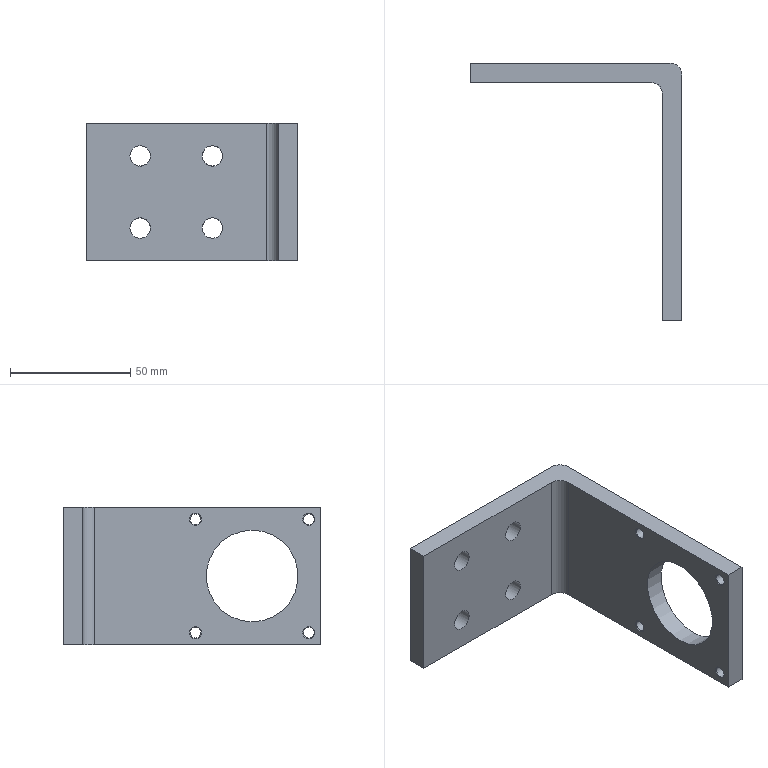Part | NX | features SIMPLE HOLE 9, DATUM_CSYS 6, SKETCH 5, SYMBOLIC_THREAD 4, EXTRUDE 3, HOLE PACKAGE 3, BLEND 1 | 1 solid | 27 faces | box 88 x 107 x 57 mm | volume 73823 mm3 | cylinder 11 | plane 8 | cone 8 | commonest cylinder face diameters 4.5 x4 8.5 x4 10 x2 38.1 x1
STEP:
#1=CARTESIAN_POINT('',(-4.,28.5,9.45));
#2=VERTEX_POINT('',#1);
#3=CARTESIAN_POINT('',(-4.,28.5,28.5));
#4=DIRECTION('',(1.,0.,0.));
#5=DIRECTION('',(0.,0.,-1.));
#6=AXIS2_PLACEMENT_3D('',#3,#4,#5);
#7=CIRCLE('',#6,19.05);
#8=EDGE_CURVE('',#2,#2,#7,.T.);
#9=ORIENTED_EDGE('',*,*,#8,.T.);
#10=EDGE_LOOP('',(#9));
#11=FACE_BOUND('',#10,.T.);
#12=CARTESIAN_POINT('',(-4.,52.05,49.55));
#13=VERTEX_POINT('',#12);
#14=CARTESIAN_POINT('',(-4.,52.05,52.05));
#15=DIRECTION('',(1.,0.,0.));
#16=DIRECTION('',(0.,0.,-1.));
#17=AXIS2_PLACEMENT_3D('',#14,#15,#16);
#18=CIRCLE('',#17,2.5);
#19=EDGE_CURVE('',#13,#13,#18,.T.);
#20=ORIENTED_EDGE('',*,*,#19,.T.);
#21=EDGE_LOOP('',(#20));
#22=FACE_BOUND('',#21,.T.);
#23=CARTESIAN_POINT('',(-4.,52.05,2.45));
#24=VERTEX_POINT('',#23);
#25=CARTESIAN_POINT('',(-4.,52.05,4.95));
#26=DIRECTION('',(1.,0.,0.));
#27=DIRECTION('',(0.,0.,-1.));
#28=AXIS2_PLACEMENT_3D('',#25,#26,#27);
#29=CIRCLE('',#28,2.5);
#30=EDGE_CURVE('',#24,#24,#29,.T.);
#31=ORIENTED_EDGE('',*,*,#30,.T.);
#32=EDGE_LOOP('',(#31));
#33=FACE_BOUND('',#32,.T.);
#34=CARTESIAN_POINT('',(-4.,4.95,49.55));
#35=VERTEX_POINT('',#34);
#36=CARTESIAN_POINT('',(-4.,4.95,52.05));
#37=DIRECTION('',(1.,0.,0.));
#38=DIRECTION('',(0.,0.,-1.));
#39=AXIS2_PLACEMENT_3D('',#36,#37,#38);
#40=CIRCLE('',#39,2.5);
#41=EDGE_CURVE('',#35,#35,#40,.T.);
#42=ORIENTED_EDGE('',*,*,#41,.T.);
#43=EDGE_LOOP('',(#42));
#44=FACE_BOUND('',#43,.T.);
#45=CARTESIAN_POINT('',(-4.,4.95,2.45));
#46=VERTEX_POINT('',#45);
#47=CARTESIAN_POINT('',(-4.,4.95,4.95));
#48=DIRECTION('',(1.,0.,0.));
#49=DIRECTION('',(0.,0.,-1.));
#50=AXIS2_PLACEMENT_3D('',#47,#48,#49);
#51=CIRCLE('',#50,2.5);
#52=EDGE_CURVE('',#46,#46,#51,.T.);
#53=ORIENTED_EDGE('',*,*,#52,.T.);
#54=EDGE_LOOP('',(#53));
#55=FACE_BOUND('',#54,.T.);
#56=CARTESIAN_POINT('',(-4.,94.,57.));
#57=VERTEX_POINT('',#56);
#58=CARTESIAN_POINT('',(-4.,0.,57.));
#59=VERTEX_POINT('',#58);
#60=CARTESIAN_POINT('',(-4.,57.,57.));
#61=DIRECTION('',(0.,-1.,0.));
#62=VECTOR('',#61,1000.);
#63=LINE('',#60,#62);
#64=EDGE_CURVE('',#57,#59,#63,.T.);
#65=ORIENTED_EDGE('',*,*,#64,.F.);
#66=CARTESIAN_POINT('',(-4.,94.,0.));
#67=VERTEX_POINT('',#66);
#68=CARTESIAN_POINT('',(-4.,94.,0.));
#69=DIRECTION('',(0.,0.,1.));
#70=VECTOR('',#69,1000.);
#71=LINE('',#68,#70);
#72=EDGE_CURVE('',#57,#67,#71,.F.);
#73=ORIENTED_EDGE('',*,*,#72,.T.);
#74=CARTESIAN_POINT('',(-4.,0.,0.));
#75=VERTEX_POINT('',#74);
#76=CARTESIAN_POINT('',(-4.,57.,0.));
#77=DIRECTION('',(0.,1.,0.));
#78=VECTOR('',#77,1000.);
#79=LINE('',#76,#78);
#80=EDGE_CURVE('',#75,#67,#79,.T.);
#81=ORIENTED_EDGE('',*,*,#80,.F.);
#82=CARTESIAN_POINT('',(-4.,0.,57.));
#83=DIRECTION('',(0.,0.,-1.));
#84=VECTOR('',#83,1000.);
#85=LINE('',#82,#84);
#86=EDGE_CURVE('',#59,#75,#85,.T.);
#87=ORIENTED_EDGE('',*,*,#86,.F.);
#88=EDGE_LOOP('',(#65,#73,#81,#87));
#89=FACE_BOUND('',#88,.T.);
#90=CARTESIAN_POINT('',(-4.,0.,0.));
#91=DIRECTION('',(1.,0.,0.));
#92=DIRECTION('',(0.,0.,-1.));
#93=AXIS2_PLACEMENT_3D('',#90,#91,#92);
#94=PLANE('',#93);
#95=ADVANCED_FACE('',(#11,#22,#33,#44,#55,#89),#94,.F.);
#96=ORIENTED_EDGE('',*,*,#86,.T.);
#97=CARTESIAN_POINT('',(4.,0.,0.));
#98=VERTEX_POINT('',#97);
#99=CARTESIAN_POINT('',(4.,0.,0.));
#100=DIRECTION('',(-1.,0.,0.));
#101=VECTOR('',#100,1000.);
#102=LINE('',#99,#101);
#103=EDGE_CURVE('',#98,#75,#102,.T.);
#104=ORIENTED_EDGE('',*,*,#103,.F.);
#105=CARTESIAN_POINT('',(4.,0.,57.));
#106=VERTEX_POINT('',#105);
#107=CARTESIAN_POINT('',(4.,0.,57.));
#108=DIRECTION('',(0.,0.,-1.));
#109=VECTOR('',#108,1000.);
#110=LINE('',#107,#109);
#111=EDGE_CURVE('',#106,#98,#110,.T.);
#112=ORIENTED_EDGE('',*,*,#111,.F.);
#113=CARTESIAN_POINT('',(4.,0.,57.));
#114=DIRECTION('',(-1.,0.,0.));
#115=VECTOR('',#114,1000.);
#116=LINE('',#113,#115);
#117=EDGE_CURVE('',#106,#59,#116,.T.);
#118=ORIENTED_EDGE('',*,*,#117,.T.);
#119=EDGE_LOOP('',(#96,#104,#112,#118));
#120=FACE_BOUND('',#119,.T.);
#121=CARTESIAN_POINT('',(4.,0.,57.));
#122=DIRECTION('',(0.,1.,0.));
#123=DIRECTION('',(0.,0.,1.));
#124=AXIS2_PLACEMENT_3D('',#121,#122,#123);
#125=PLANE('',#124);
#126=ADVANCED_FACE('',(#120),#125,.F.);
#127=CARTESIAN_POINT('',(-1.,107.,0.));
#128=VERTEX_POINT('',#127);
#129=CARTESIAN_POINT('',(-84.,107.,0.));
#130=VERTEX_POINT('',#129);
#131=CARTESIAN_POINT('',(4.,107.,0.));
#132=DIRECTION('',(-1.,0.,0.));
#133=VECTOR('',#132,1000.);
#134=LINE('',#131,#133);
#135=EDGE_CURVE('',#128,#130,#134,.T.);
#136=ORIENTED_EDGE('',*,*,#135,.F.);
#137=CARTESIAN_POINT('',(4.,102.,0.));
#138=VERTEX_POINT('',#137);
#139=CARTESIAN_POINT('',(-1.,102.,0.));
#140=DIRECTION('',(0.,0.,1.));
#141=DIRECTION('',(0.,-1.,0.));
#142=AXIS2_PLACEMENT_3D('',#139,#140,#141);
#143=CIRCLE('',#142,5.);
#144=EDGE_CURVE('',#128,#138,#143,.F.);
#145=ORIENTED_EDGE('',*,*,#144,.T.);
#146=CARTESIAN_POINT('',(4.,0.,0.));
#147=DIRECTION('',(0.,1.,0.));
#148=VECTOR('',#147,1000.);
#149=LINE('',#146,#148);
#150=EDGE_CURVE('',#98,#138,#149,.T.);
#151=ORIENTED_EDGE('',*,*,#150,.F.);
#152=ORIENTED_EDGE('',*,*,#103,.T.);
#153=ORIENTED_EDGE('',*,*,#80,.T.);
#154=CARTESIAN_POINT('',(-9.,99.,0.));
#155=VERTEX_POINT('',#154);
#156=CARTESIAN_POINT('',(-9.,94.,0.));
#157=DIRECTION('',(0.,0.,1.));
#158=DIRECTION('',(0.,-1.,0.));
#159=AXIS2_PLACEMENT_3D('',#156,#157,#158);
#160=CIRCLE('',#159,5.);
#161=EDGE_CURVE('',#67,#155,#160,.T.);
#162=ORIENTED_EDGE('',*,*,#161,.T.);
#163=CARTESIAN_POINT('',(-84.,99.,0.));
#164=VERTEX_POINT('',#163);
#165=CARTESIAN_POINT('',(-84.,99.,0.));
#166=DIRECTION('',(-1.,0.,0.));
#167=VECTOR('',#166,1000.);
#168=LINE('',#165,#167);
#169=EDGE_CURVE('',#155,#164,#168,.T.);
#170=ORIENTED_EDGE('',*,*,#169,.T.);
#171=CARTESIAN_POINT('',(-84.,107.,0.));
#172=DIRECTION('',(0.,1.,0.));
#173=VECTOR('',#172,1000.);
#174=LINE('',#171,#173);
#175=EDGE_CURVE('',#164,#130,#174,.T.);
#176=ORIENTED_EDGE('',*,*,#175,.T.);
#177=EDGE_LOOP('',(#136,#145,#151,#152,#153,#162,#170,#176));
#178=FACE_BOUND('',#177,.T.);
#179=CARTESIAN_POINT('',(4.,57.,0.));
#180=DIRECTION('',(0.,0.,1.));
#181=DIRECTION('',(0.,-1.,0.));
#182=AXIS2_PLACEMENT_3D('',#179,#180,#181);
#183=PLANE('',#182);
#184=ADVANCED_FACE('',(#178),#183,.F.);
#185=CARTESIAN_POINT('',(-31.5,107.,9.25));
#186=VERTEX_POINT('',#185);
#187=CARTESIAN_POINT('',(-31.5,107.,13.5));
#188=DIRECTION('',(0.,-1.,0.));
#189=DIRECTION('',(0.,0.,-1.));
#190=AXIS2_PLACEMENT_3D('',#187,#188,#189);
#191=CIRCLE('',#190,4.25);
#192=EDGE_CURVE('',#186,#186,#191,.T.);
#193=ORIENTED_EDGE('',*,*,#192,.T.);
#194=EDGE_LOOP('',(#193));
#195=FACE_BOUND('',#194,.T.);
#196=CARTESIAN_POINT('',(-61.5,107.,9.25));
#197=VERTEX_POINT('',#196);
#198=CARTESIAN_POINT('',(-61.5,107.,13.5));
#199=DIRECTION('',(0.,-1.,0.));
#200=DIRECTION('',(0.,0.,-1.));
#201=AXIS2_PLACEMENT_3D('',#198,#199,#200);
#202=CIRCLE('',#201,4.25);
#203=EDGE_CURVE('',#197,#197,#202,.T.);
#204=ORIENTED_EDGE('',*,*,#203,.T.);
#205=EDGE_LOOP('',(#204));
#206=FACE_BOUND('',#205,.T.);
#207=CARTESIAN_POINT('',(-61.5,107.,39.25));
#208=VERTEX_POINT('',#207);
#209=CARTESIAN_POINT('',(-61.5,107.,43.5));
#210=DIRECTION('',(0.,-1.,0.));
#211=DIRECTION('',(0.,0.,-1.));
#212=AXIS2_PLACEMENT_3D('',#209,#210,#211);
#213=CIRCLE('',#212,4.25);
#214=EDGE_CURVE('',#208,#208,#213,.T.);
#215=ORIENTED_EDGE('',*,*,#214,.T.);
#216=EDGE_LOOP('',(#215));
#217=FACE_BOUND('',#216,.T.);
#218=CARTESIAN_POINT('',(-31.5,107.,39.25));
#219=VERTEX_POINT('',#218);
#220=CARTESIAN_POINT('',(-31.5,107.,43.5));
#221=DIRECTION('',(0.,-1.,0.));
#222=DIRECTION('',(0.,0.,-1.));
#223=AXIS2_PLACEMENT_3D('',#220,#221,#222);
#224=CIRCLE('',#223,4.25);
#225=EDGE_CURVE('',#219,#219,#224,.T.);
#226=ORIENTED_EDGE('',*,*,#225,.T.);
#227=EDGE_LOOP('',(#226));
#228=FACE_BOUND('',#227,.T.);
#229=CARTESIAN_POINT('',(-84.,107.,57.));
#230=VERTEX_POINT('',#229);
#231=CARTESIAN_POINT('',(-1.,107.,57.));
#232=VERTEX_POINT('',#231);
#233=CARTESIAN_POINT('',(4.,107.,57.));
#234=DIRECTION('',(1.,0.,0.));
#235=VECTOR('',#234,1000.);
#236=LINE('',#233,#235);
#237=EDGE_CURVE('',#230,#232,#236,.T.);
#238=ORIENTED_EDGE('',*,*,#237,.T.);
#239=CARTESIAN_POINT('',(-1.,107.,0.));
#240=DIRECTION('',(0.,0.,1.));
#241=VECTOR('',#240,1000.);
#242=LINE('',#239,#241);
#243=EDGE_CURVE('',#232,#128,#242,.F.);
#244=ORIENTED_EDGE('',*,*,#243,.T.);
#245=ORIENTED_EDGE('',*,*,#135,.T.);
#246=CARTESIAN_POINT('',(-84.,107.,-467.25));
#247=DIRECTION('',(0.,0.,1.));
#248=VECTOR('',#247,1000.);
#249=LINE('',#246,#248);
#250=EDGE_CURVE('',#130,#230,#249,.T.);
#251=ORIENTED_EDGE('',*,*,#250,.T.);
#252=EDGE_LOOP('',(#238,#244,#245,#251));
#253=FACE_BOUND('',#252,.T.);
#254=CARTESIAN_POINT('',(4.,107.,0.));
#255=DIRECTION('',(0.,-1.,0.));
#256=DIRECTION('',(0.,0.,-1.));
#257=AXIS2_PLACEMENT_3D('',#254,#255,#256);
#258=PLANE('',#257);
#259=ADVANCED_FACE('',(#195,#206,#217,#228,#253),#258,.F.);
#260=CARTESIAN_POINT('',(4.,102.,57.));
#261=VERTEX_POINT('',#260);
#262=CARTESIAN_POINT('',(4.,57.,57.));
#263=DIRECTION('',(0.,-1.,0.));
#264=VECTOR('',#263,1000.);
#265=LINE('',#262,#264);
#266=EDGE_CURVE('',#261,#106,#265,.T.);
#267=ORIENTED_EDGE('',*,*,#266,.F.);
#268=CARTESIAN_POINT('',(-1.,102.,57.));
#269=DIRECTION('',(0.,0.,-1.));
#270=DIRECTION('',(-1.,0.,0.));
#271=AXIS2_PLACEMENT_3D('',#268,#269,#270);
#272=CIRCLE('',#271,5.);
#273=EDGE_CURVE('',#261,#232,#272,.F.);
#274=ORIENTED_EDGE('',*,*,#273,.T.);
#275=ORIENTED_EDGE('',*,*,#237,.F.);
#276=CARTESIAN_POINT('',(-84.,99.,57.));
#277=VERTEX_POINT('',#276);
#278=CARTESIAN_POINT('',(-84.,107.,57.));
#279=DIRECTION('',(0.,1.,0.));
#280=VECTOR('',#279,1000.);
#281=LINE('',#278,#280);
#282=EDGE_CURVE('',#277,#230,#281,.T.);
#283=ORIENTED_EDGE('',*,*,#282,.F.);
#284=CARTESIAN_POINT('',(-9.,99.,57.));
#285=VERTEX_POINT('',#284);
#286=CARTESIAN_POINT('',(-84.,99.,57.));
#287=DIRECTION('',(-1.,0.,0.));
#288=VECTOR('',#287,1000.);
#289=LINE('',#286,#288);
#290=EDGE_CURVE('',#285,#277,#289,.T.);
#291=ORIENTED_EDGE('',*,*,#290,.F.);
#292=CARTESIAN_POINT('',(-9.,94.,57.));
#293=DIRECTION('',(0.,0.,-1.));
#294=DIRECTION('',(-1.,0.,0.));
#295=AXIS2_PLACEMENT_3D('',#292,#293,#294);
#296=CIRCLE('',#295,5.);
#297=EDGE_CURVE('',#285,#57,#296,.T.);
#298=ORIENTED_EDGE('',*,*,#297,.T.);
#299=ORIENTED_EDGE('',*,*,#64,.T.);
#300=ORIENTED_EDGE('',*,*,#117,.F.);
#301=EDGE_LOOP('',(#267,#274,#275,#283,#291,#298,#299,#300));
#302=FACE_BOUND('',#301,.T.);
#303=CARTESIAN_POINT('',(4.,57.,57.));
#304=DIRECTION('',(0.,0.,-1.));
#305=DIRECTION('',(-1.,0.,0.));
#306=AXIS2_PLACEMENT_3D('',#303,#304,#305);
#307=PLANE('',#306);
#308=ADVANCED_FACE('',(#302),#307,.F.);
#309=CARTESIAN_POINT('',(4.,28.5,47.55));
#310=VERTEX_POINT('',#309);
#311=CARTESIAN_POINT('',(4.,28.5,28.5));
#312=DIRECTION('',(-1.,0.,0.));
#313=DIRECTION('',(0.,0.,1.));
#314=AXIS2_PLACEMENT_3D('',#311,#312,#313);
#315=CIRCLE('',#314,19.05);
#316=EDGE_CURVE('',#310,#310,#315,.T.);
#317=ORIENTED_EDGE('',*,*,#316,.T.);
#318=EDGE_LOOP('',(#317));
#319=FACE_BOUND('',#318,.T.);
#320=CARTESIAN_POINT('',(4.,52.05,49.55));
#321=VERTEX_POINT('',#320);
#322=CARTESIAN_POINT('',(4.,52.05,52.05));
#323=DIRECTION('',(1.,0.,0.));
#324=DIRECTION('',(0.,0.,-1.));
#325=AXIS2_PLACEMENT_3D('',#322,#323,#324);
#326=CIRCLE('',#325,2.5);
#327=EDGE_CURVE('',#321,#321,#326,.F.);
#328=ORIENTED_EDGE('',*,*,#327,.T.);
#329=EDGE_LOOP('',(#328));
#330=FACE_BOUND('',#329,.T.);
#331=CARTESIAN_POINT('',(4.,52.05,2.45));
#332=VERTEX_POINT('',#331);
#333=CARTESIAN_POINT('',(4.,52.05,4.95));
#334=DIRECTION('',(1.,0.,0.));
#335=DIRECTION('',(0.,0.,-1.));
#336=AXIS2_PLACEMENT_3D('',#333,#334,#335);
#337=CIRCLE('',#336,2.5);
#338=EDGE_CURVE('',#332,#332,#337,.F.);
#339=ORIENTED_EDGE('',*,*,#338,.T.);
#340=EDGE_LOOP('',(#339));
#341=FACE_BOUND('',#340,.T.);
#342=CARTESIAN_POINT('',(4.,4.95,49.55));
#343=VERTEX_POINT('',#342);
#344=CARTESIAN_POINT('',(4.,4.95,52.05));
#345=DIRECTION('',(1.,0.,0.));
#346=DIRECTION('',(0.,0.,-1.));
#347=AXIS2_PLACEMENT_3D('',#344,#345,#346);
#348=CIRCLE('',#347,2.5);
#349=EDGE_CURVE('',#343,#343,#348,.F.);
#350=ORIENTED_EDGE('',*,*,#349,.T.);
#351=EDGE_LOOP('',(#350));
#352=FACE_BOUND('',#351,.T.);
#353=CARTESIAN_POINT('',(4.,4.95,2.45));
#354=VERTEX_POINT('',#353);
#355=CARTESIAN_POINT('',(4.,4.95,4.95));
#356=DIRECTION('',(1.,0.,0.));
#357=DIRECTION('',(0.,0.,-1.));
#358=AXIS2_PLACEMENT_3D('',#355,#356,#357);
#359=CIRCLE('',#358,2.5);
#360=EDGE_CURVE('',#354,#354,#359,.F.);
#361=ORIENTED_EDGE('',*,*,#360,.T.);
#362=EDGE_LOOP('',(#361));
#363=FACE_BOUND('',#362,.T.);
#364=ORIENTED_EDGE('',*,*,#150,.T.);
#365=CARTESIAN_POINT('',(4.,102.,57.));
#366=DIRECTION('',(0.,0.,1.));
#367=VECTOR('',#366,1000.);
#368=LINE('',#365,#367);
#369=EDGE_CURVE('',#138,#261,#368,.T.);
#370=ORIENTED_EDGE('',*,*,#369,.T.);
#371=ORIENTED_EDGE('',*,*,#266,.T.);
#372=ORIENTED_EDGE('',*,*,#111,.T.);
#373=EDGE_LOOP('',(#364,#370,#371,#372));
#374=FACE_BOUND('',#373,.T.);
#375=CARTESIAN_POINT('',(4.,0.,0.));
#376=DIRECTION('',(1.,0.,0.));
#377=DIRECTION('',(0.,0.,-1.));
#378=AXIS2_PLACEMENT_3D('',#375,#376,#377);
#379=PLANE('',#378);
#380=ADVANCED_FACE('',(#319,#330,#341,#352,#363,#374),#379,.T.);
#381=CARTESIAN_POINT('',(-35.75,99.,13.5));
#382=VERTEX_POINT('',#381);
#383=CARTESIAN_POINT('',(-31.5,99.,13.5));
#384=DIRECTION('',(0.,1.,0.));
#385=DIRECTION('',(-1.,0.,0.));
#386=AXIS2_PLACEMENT_3D('',#383,#384,#385);
#387=CIRCLE('',#386,4.25);
#388=EDGE_CURVE('',#382,#382,#387,.T.);
#389=ORIENTED_EDGE('',*,*,#388,.T.);
#390=EDGE_LOOP('',(#389));
#391=FACE_BOUND('',#390,.T.);
#392=CARTESIAN_POINT('',(-65.75,99.,13.5));
#393=VERTEX_POINT('',#392);
#394=CARTESIAN_POINT('',(-61.5,99.,13.5));
#395=DIRECTION('',(0.,1.,0.));
#396=DIRECTION('',(-1.,0.,0.));
#397=AXIS2_PLACEMENT_3D('',#394,#395,#396);
#398=CIRCLE('',#397,4.25);
#399=EDGE_CURVE('',#393,#393,#398,.T.);
#400=ORIENTED_EDGE('',*,*,#399,.T.);
#401=EDGE_LOOP('',(#400));
#402=FACE_BOUND('',#401,.T.);
#403=CARTESIAN_POINT('',(-65.75,99.,43.5));
#404=VERTEX_POINT('',#403);
#405=CARTESIAN_POINT('',(-61.5,99.,43.5));
#406=DIRECTION('',(0.,1.,0.));
#407=DIRECTION('',(-1.,0.,0.));
#408=AXIS2_PLACEMENT_3D('',#405,#406,#407);
#409=CIRCLE('',#408,4.25);
#410=EDGE_CURVE('',#404,#404,#409,.T.);
#411=ORIENTED_EDGE('',*,*,#410,.T.);
#412=EDGE_LOOP('',(#411));
#413=FACE_BOUND('',#412,.T.);
#414=CARTESIAN_POINT('',(-35.75,99.,43.5));
#415=VERTEX_POINT('',#414);
#416=CARTESIAN_POINT('',(-31.5,99.,43.5));
#417=DIRECTION('',(0.,1.,0.));
#418=DIRECTION('',(-1.,0.,0.));
#419=AXIS2_PLACEMENT_3D('',#416,#417,#418);
#420=CIRCLE('',#419,4.25);
#421=EDGE_CURVE('',#415,#415,#420,.T.);
#422=ORIENTED_EDGE('',*,*,#421,.T.);
#423=EDGE_LOOP('',(#422));
#424=FACE_BOUND('',#423,.T.);
#425=ORIENTED_EDGE('',*,*,#169,.F.);
#426=CARTESIAN_POINT('',(-9.,99.,-467.25));
#427=DIRECTION('',(0.,0.,1.));
#428=VECTOR('',#427,1000.);
#429=LINE('',#426,#428);
#430=EDGE_CURVE('',#155,#285,#429,.T.);
#431=ORIENTED_EDGE('',*,*,#430,.T.);
#432=ORIENTED_EDGE('',*,*,#290,.T.);
#433=CARTESIAN_POINT('',(-84.,99.,-467.25));
#434=DIRECTION('',(0.,0.,1.));
#435=VECTOR('',#434,1000.);
#436=LINE('',#433,#435);
#437=EDGE_CURVE('',#164,#277,#436,.T.);
#438=ORIENTED_EDGE('',*,*,#437,.F.);
#439=EDGE_LOOP('',(#425,#431,#432,#438));
#440=FACE_BOUND('',#439,.T.);
#441=CARTESIAN_POINT('',(-84.,99.,-467.25));
#442=DIRECTION('',(0.,-1.,0.));
#443=DIRECTION('',(1.,0.,0.));
#444=AXIS2_PLACEMENT_3D('',#441,#442,#443);
#445=PLANE('',#444);
#446=ADVANCED_FACE('',(#391,#402,#413,#424,#440),#445,.T.);
#447=ORIENTED_EDGE('',*,*,#175,.F.);
#448=ORIENTED_EDGE('',*,*,#437,.T.);
#449=ORIENTED_EDGE('',*,*,#282,.T.);
#450=ORIENTED_EDGE('',*,*,#250,.F.);
#451=EDGE_LOOP('',(#447,#448,#449,#450));
#452=FACE_BOUND('',#451,.T.);
#453=CARTESIAN_POINT('',(-84.,107.,-467.25));
#454=DIRECTION('',(-1.,0.,0.));
#455=DIRECTION('',(0.,0.,1.));
#456=AXIS2_PLACEMENT_3D('',#453,#454,#455);
#457=PLANE('',#456);
#458=ADVANCED_FACE('',(#452),#457,.T.);
#459=ORIENTED_EDGE('',*,*,#144,.F.);
#460=ORIENTED_EDGE('',*,*,#243,.F.);
#461=ORIENTED_EDGE('',*,*,#273,.F.);
#462=ORIENTED_EDGE('',*,*,#369,.F.);
#463=EDGE_LOOP('',(#459,#460,#461,#462));
#464=FACE_BOUND('',#463,.T.);
#465=CARTESIAN_POINT('',(-1.,102.,0.));
#466=DIRECTION('',(0.,0.,-1.));
#467=DIRECTION('',(0.,1.,0.));
#468=AXIS2_PLACEMENT_3D('',#465,#466,#467);
#469=CYLINDRICAL_SURFACE('',#468,5.);
#470=ADVANCED_FACE('',(#464),#469,.T.);
#471=ORIENTED_EDGE('',*,*,#161,.F.);
#472=ORIENTED_EDGE('',*,*,#72,.F.);
#473=ORIENTED_EDGE('',*,*,#297,.F.);
#474=ORIENTED_EDGE('',*,*,#430,.F.);
#475=EDGE_LOOP('',(#471,#472,#473,#474));
#476=FACE_BOUND('',#475,.T.);
#477=CARTESIAN_POINT('',(-9.,94.,-467.25));
#478=DIRECTION('',(0.,0.,1.));
#479=DIRECTION('',(1.,0.,0.));
#480=AXIS2_PLACEMENT_3D('',#477,#478,#479);
#481=CYLINDRICAL_SURFACE('',#480,5.);
#482=ADVANCED_FACE('',(#476),#481,.F.);
#483=CARTESIAN_POINT('',(3.75,4.95,2.7));
#484=VERTEX_POINT('',#483);
#485=CARTESIAN_POINT('',(3.75,4.95,4.95));
#486=DIRECTION('',(1.,0.,0.));
#487=DIRECTION('',(0.,0.,-1.));
#488=AXIS2_PLACEMENT_3D('',#485,#486,#487);
#489=CIRCLE('',#488,2.25);
#490=EDGE_CURVE('',#484,#484,#489,.T.);
#491=ORIENTED_EDGE('',*,*,#490,.T.);
#492=EDGE_LOOP('',(#491));
#493=FACE_BOUND('',#492,.T.);
#494=CARTESIAN_POINT('',(-3.75,4.95,2.7));
#495=VERTEX_POINT('',#494);
#496=CARTESIAN_POINT('',(-3.75,4.95,4.95));
#497=DIRECTION('',(1.,0.,0.));
#498=DIRECTION('',(0.,0.,-1.));
#499=AXIS2_PLACEMENT_3D('',#496,#497,#498);
#500=CIRCLE('',#499,2.25);
#501=EDGE_CURVE('',#495,#495,#500,.F.);
#502=ORIENTED_EDGE('',*,*,#501,.T.);
#503=EDGE_LOOP('',(#502));
#504=FACE_BOUND('',#503,.T.);
#505=CARTESIAN_POINT('',(-4.,4.95,4.95));
#506=DIRECTION('',(1.,0.,0.));
#507=DIRECTION('',(0.,0.,-1.));
#508=AXIS2_PLACEMENT_3D('',#505,#506,#507);
#509=CYLINDRICAL_SURFACE('',#508,2.25);
#510=ADVANCED_FACE('',(#493,#504),#509,.F.);
#511=ORIENTED_EDGE('',*,*,#501,.F.);
#512=EDGE_LOOP('',(#511));
#513=FACE_BOUND('',#512,.T.);
#514=ORIENTED_EDGE('',*,*,#52,.F.);
#515=EDGE_LOOP('',(#514));
#516=FACE_BOUND('',#515,.T.);
#517=CARTESIAN_POINT('',(-4.,4.95,4.95));
#518=DIRECTION('',(-1.,0.,0.));
#519=DIRECTION('',(0.,0.,1.));
#520=AXIS2_PLACEMENT_3D('',#517,#518,#519);
#521=CONICAL_SURFACE('',#520,2.5,0.7854);
#522=ADVANCED_FACE('',(#513,#516),#521,.F.);
#523=ORIENTED_EDGE('',*,*,#360,.F.);
#524=EDGE_LOOP('',(#523));
#525=FACE_BOUND('',#524,.T.);
#526=ORIENTED_EDGE('',*,*,#490,.F.);
#527=EDGE_LOOP('',(#526));
#528=FACE_BOUND('',#527,.T.);
#529=CARTESIAN_POINT('',(3.75,4.95,4.95));
#530=DIRECTION('',(1.,0.,0.));
#531=DIRECTION('',(0.,0.,-1.));
#532=AXIS2_PLACEMENT_3D('',#529,#530,#531);
#533=CONICAL_SURFACE('',#532,2.25,0.7854);
#534=ADVANCED_FACE('',(#525,#528),#533,.F.);
#535=CARTESIAN_POINT('',(3.75,4.95,49.8));
#536=VERTEX_POINT('',#535);
#537=CARTESIAN_POINT('',(3.75,4.95,52.05));
#538=DIRECTION('',(1.,0.,0.));
#539=DIRECTION('',(0.,0.,-1.));
#540=AXIS2_PLACEMENT_3D('',#537,#538,#539);
#541=CIRCLE('',#540,2.25);
#542=EDGE_CURVE('',#536,#536,#541,.T.);
#543=ORIENTED_EDGE('',*,*,#542,.T.);
#544=EDGE_LOOP('',(#543));
#545=FACE_BOUND('',#544,.T.);
#546=CARTESIAN_POINT('',(-3.75,4.95,49.8));
#547=VERTEX_POINT('',#546);
#548=CARTESIAN_POINT('',(-3.75,4.95,52.05));
#549=DIRECTION('',(1.,0.,0.));
#550=DIRECTION('',(0.,0.,-1.));
#551=AXIS2_PLACEMENT_3D('',#548,#549,#550);
#552=CIRCLE('',#551,2.25);
#553=EDGE_CURVE('',#547,#547,#552,.F.);
#554=ORIENTED_EDGE('',*,*,#553,.T.);
#555=EDGE_LOOP('',(#554));
#556=FACE_BOUND('',#555,.T.);
#557=CARTESIAN_POINT('',(-4.,4.95,52.05));
#558=DIRECTION('',(1.,0.,0.));
#559=DIRECTION('',(0.,0.,-1.));
#560=AXIS2_PLACEMENT_3D('',#557,#558,#559);
#561=CYLINDRICAL_SURFACE('',#560,2.25);
#562=ADVANCED_FACE('',(#545,#556),#561,.F.);
#563=ORIENTED_EDGE('',*,*,#553,.F.);
#564=EDGE_LOOP('',(#563));
#565=FACE_BOUND('',#564,.T.);
#566=ORIENTED_EDGE('',*,*,#41,.F.);
#567=EDGE_LOOP('',(#566));
#568=FACE_BOUND('',#567,.T.);
#569=CARTESIAN_POINT('',(-4.,4.95,52.05));
#570=DIRECTION('',(-1.,0.,0.));
#571=DIRECTION('',(0.,0.,1.));
#572=AXIS2_PLACEMENT_3D('',#569,#570,#571);
#573=CONICAL_SURFACE('',#572,2.5,0.7854);
#574=ADVANCED_FACE('',(#565,#568),#573,.F.);
#575=ORIENTED_EDGE('',*,*,#349,.F.);
#576=EDGE_LOOP('',(#575));
#577=FACE_BOUND('',#576,.T.);
#578=ORIENTED_EDGE('',*,*,#542,.F.);
#579=EDGE_LOOP('',(#578));
#580=FACE_BOUND('',#579,.T.);
#581=CARTESIAN_POINT('',(3.75,4.95,52.05));
#582=DIRECTION('',(1.,0.,0.));
#583=DIRECTION('',(0.,0.,-1.));
#584=AXIS2_PLACEMENT_3D('',#581,#582,#583);
#585=CONICAL_SURFACE('',#584,2.25,0.7854);
#586=ADVANCED_FACE('',(#577,#580),#585,.F.);
#587=CARTESIAN_POINT('',(3.75,52.05,2.7));
#588=VERTEX_POINT('',#587);
#589=CARTESIAN_POINT('',(3.75,52.05,4.95));
#590=DIRECTION('',(1.,0.,0.));
#591=DIRECTION('',(0.,0.,-1.));
#592=AXIS2_PLACEMENT_3D('',#589,#590,#591);
#593=CIRCLE('',#592,2.25);
#594=EDGE_CURVE('',#588,#588,#593,.T.);
#595=ORIENTED_EDGE('',*,*,#594,.T.);
#596=EDGE_LOOP('',(#595));
#597=FACE_BOUND('',#596,.T.);
#598=CARTESIAN_POINT('',(-3.75,52.05,2.7));
#599=VERTEX_POINT('',#598);
#600=CARTESIAN_POINT('',(-3.75,52.05,4.95));
#601=DIRECTION('',(1.,0.,0.));
#602=DIRECTION('',(0.,0.,-1.));
#603=AXIS2_PLACEMENT_3D('',#600,#601,#602);
#604=CIRCLE('',#603,2.25);
#605=EDGE_CURVE('',#599,#599,#604,.F.);
#606=ORIENTED_EDGE('',*,*,#605,.T.);
#607=EDGE_LOOP('',(#606));
#608=FACE_BOUND('',#607,.T.);
#609=CARTESIAN_POINT('',(-4.,52.05,4.95));
#610=DIRECTION('',(1.,0.,0.));
#611=DIRECTION('',(0.,0.,-1.));
#612=AXIS2_PLACEMENT_3D('',#609,#610,#611);
#613=CYLINDRICAL_SURFACE('',#612,2.25);
#614=ADVANCED_FACE('',(#597,#608),#613,.F.);
#615=ORIENTED_EDGE('',*,*,#605,.F.);
#616=EDGE_LOOP('',(#615));
#617=FACE_BOUND('',#616,.T.);
#618=ORIENTED_EDGE('',*,*,#30,.F.);
#619=EDGE_LOOP('',(#618));
#620=FACE_BOUND('',#619,.T.);
#621=CARTESIAN_POINT('',(-4.,52.05,4.95));
#622=DIRECTION('',(-1.,0.,0.));
#623=DIRECTION('',(0.,0.,1.));
#624=AXIS2_PLACEMENT_3D('',#621,#622,#623);
#625=CONICAL_SURFACE('',#624,2.5,0.7854);
#626=ADVANCED_FACE('',(#617,#620),#625,.F.);
#627=ORIENTED_EDGE('',*,*,#338,.F.);
#628=EDGE_LOOP('',(#627));
#629=FACE_BOUND('',#628,.T.);
#630=ORIENTED_EDGE('',*,*,#594,.F.);
#631=EDGE_LOOP('',(#630));
#632=FACE_BOUND('',#631,.T.);
#633=CARTESIAN_POINT('',(3.75,52.05,4.95));
#634=DIRECTION('',(1.,0.,0.));
#635=DIRECTION('',(0.,0.,-1.));
#636=AXIS2_PLACEMENT_3D('',#633,#634,#635);
#637=CONICAL_SURFACE('',#636,2.25,0.7854);
#638=ADVANCED_FACE('',(#629,#632),#637,.F.);
#639=CARTESIAN_POINT('',(3.75,52.05,49.8));
#640=VERTEX_POINT('',#639);
#641=CARTESIAN_POINT('',(3.75,52.05,52.05));
#642=DIRECTION('',(1.,0.,0.));
#643=DIRECTION('',(0.,0.,-1.));
#644=AXIS2_PLACEMENT_3D('',#641,#642,#643);
#645=CIRCLE('',#644,2.25);
#646=EDGE_CURVE('',#640,#640,#645,.T.);
#647=ORIENTED_EDGE('',*,*,#646,.T.);
#648=EDGE_LOOP('',(#647));
#649=FACE_BOUND('',#648,.T.);
#650=CARTESIAN_POINT('',(-3.75,52.05,49.8));
#651=VERTEX_POINT('',#650);
#652=CARTESIAN_POINT('',(-3.75,52.05,52.05));
#653=DIRECTION('',(1.,0.,0.));
#654=DIRECTION('',(0.,0.,-1.));
#655=AXIS2_PLACEMENT_3D('',#652,#653,#654);
#656=CIRCLE('',#655,2.25);
#657=EDGE_CURVE('',#651,#651,#656,.F.);
#658=ORIENTED_EDGE('',*,*,#657,.T.);
#659=EDGE_LOOP('',(#658));
#660=FACE_BOUND('',#659,.T.);
#661=CARTESIAN_POINT('',(-4.,52.05,52.05));
#662=DIRECTION('',(1.,0.,0.));
#663=DIRECTION('',(0.,0.,-1.));
#664=AXIS2_PLACEMENT_3D('',#661,#662,#663);
#665=CYLINDRICAL_SURFACE('',#664,2.25);
#666=ADVANCED_FACE('',(#649,#660),#665,.F.);
#667=ORIENTED_EDGE('',*,*,#657,.F.);
#668=EDGE_LOOP('',(#667));
#669=FACE_BOUND('',#668,.T.);
#670=ORIENTED_EDGE('',*,*,#19,.F.);
#671=EDGE_LOOP('',(#670));
#672=FACE_BOUND('',#671,.T.);
#673=CARTESIAN_POINT('',(-4.,52.05,52.05));
#674=DIRECTION('',(-1.,0.,0.));
#675=DIRECTION('',(0.,0.,1.));
#676=AXIS2_PLACEMENT_3D('',#673,#674,#675);
#677=CONICAL_SURFACE('',#676,2.5,0.7854);
#678=ADVANCED_FACE('',(#669,#672),#677,.F.);
#679=ORIENTED_EDGE('',*,*,#327,.F.);
#680=EDGE_LOOP('',(#679));
#681=FACE_BOUND('',#680,.T.);
#682=ORIENTED_EDGE('',*,*,#646,.F.);
#683=EDGE_LOOP('',(#682));
#684=FACE_BOUND('',#683,.T.);
#685=CARTESIAN_POINT('',(3.75,52.05,52.05));
#686=DIRECTION('',(1.,0.,0.));
#687=DIRECTION('',(0.,0.,-1.));
#688=AXIS2_PLACEMENT_3D('',#685,#686,#687);
#689=CONICAL_SURFACE('',#688,2.25,0.7854);
#690=ADVANCED_FACE('',(#681,#684),#689,.F.);
#691=ORIENTED_EDGE('',*,*,#421,.F.);
#692=EDGE_LOOP('',(#691));
#693=FACE_BOUND('',#692,.T.);
#694=ORIENTED_EDGE('',*,*,#225,.F.);
#695=EDGE_LOOP('',(#694));
#696=FACE_BOUND('',#695,.T.);
#697=CARTESIAN_POINT('',(-31.5,99.,43.5));
#698=DIRECTION('',(0.,1.,0.));
#699=DIRECTION('',(-1.,0.,0.));
#700=AXIS2_PLACEMENT_3D('',#697,#698,#699);
#701=CYLINDRICAL_SURFACE('',#700,4.25);
#702=ADVANCED_FACE('',(#693,#696),#701,.F.);
#703=ORIENTED_EDGE('',*,*,#410,.F.);
#704=EDGE_LOOP('',(#703));
#705=FACE_BOUND('',#704,.T.);
#706=ORIENTED_EDGE('',*,*,#214,.F.);
#707=EDGE_LOOP('',(#706));
#708=FACE_BOUND('',#707,.T.);
#709=CARTESIAN_POINT('',(-61.5,99.,43.5));
#710=DIRECTION('',(0.,1.,0.));
#711=DIRECTION('',(-1.,0.,0.));
#712=AXIS2_PLACEMENT_3D('',#709,#710,#711);
#713=CYLINDRICAL_SURFACE('',#712,4.25);
#714=ADVANCED_FACE('',(#705,#708),#713,.F.);
#715=ORIENTED_EDGE('',*,*,#399,.F.);
#716=EDGE_LOOP('',(#715));
#717=FACE_BOUND('',#716,.T.);
#718=ORIENTED_EDGE('',*,*,#203,.F.);
#719=EDGE_LOOP('',(#718));
#720=FACE_BOUND('',#719,.T.);
#721=CARTESIAN_POINT('',(-61.5,99.,13.5));
#722=DIRECTION('',(0.,1.,0.));
#723=DIRECTION('',(-1.,0.,0.));
#724=AXIS2_PLACEMENT_3D('',#721,#722,#723);
#725=CYLINDRICAL_SURFACE('',#724,4.25);
#726=ADVANCED_FACE('',(#717,#720),#725,.F.);
#727=ORIENTED_EDGE('',*,*,#388,.F.);
#728=EDGE_LOOP('',(#727));
#729=FACE_BOUND('',#728,.T.);
#730=ORIENTED_EDGE('',*,*,#192,.F.);
#731=EDGE_LOOP('',(#730));
#732=FACE_BOUND('',#731,.T.);
#733=CARTESIAN_POINT('',(-31.5,99.,13.5));
#734=DIRECTION('',(0.,1.,0.));
#735=DIRECTION('',(-1.,0.,0.));
#736=AXIS2_PLACEMENT_3D('',#733,#734,#735);
#737=CYLINDRICAL_SURFACE('',#736,4.25);
#738=ADVANCED_FACE('',(#729,#732),#737,.F.);
#739=ORIENTED_EDGE('',*,*,#316,.F.);
#740=EDGE_LOOP('',(#739));
#741=FACE_BOUND('',#740,.T.);
#742=ORIENTED_EDGE('',*,*,#8,.F.);
#743=EDGE_LOOP('',(#742));
#744=FACE_BOUND('',#743,.T.);
#745=CARTESIAN_POINT('',(4.,28.5,28.5));
#746=DIRECTION('',(-1.,0.,0.));
#747=DIRECTION('',(0.,0.,1.));
#748=AXIS2_PLACEMENT_3D('',#745,#746,#747);
#749=CYLINDRICAL_SURFACE('',#748,19.05);
#750=ADVANCED_FACE('',(#741,#744),#749,.F.);
#751=CLOSED_SHELL('',(#95,#126,#184,#259,#308,#380,#446,#458,#470,#482,#510,#522,#534,#562,#574,#586,#614,#626,#638,#666,#678,#690,#702,#714,#726,#738,#750));
#752=MANIFOLD_SOLID_BREP('',#751);
#753=(LENGTH_UNIT()NAMED_UNIT(*)SI_UNIT(.MILLI.,.METRE.));
#754=UNCERTAINTY_MEASURE_WITH_UNIT(LENGTH_MEASURE(0.00001),#753,'','');
#755=(NAMED_UNIT(*)PLANE_ANGLE_UNIT()SI_UNIT($,.RADIAN.));
#756=(NAMED_UNIT(*)SI_UNIT($,.STERADIAN.)SOLID_ANGLE_UNIT());
#757=(GEOMETRIC_REPRESENTATION_CONTEXT(3)GLOBAL_UNCERTAINTY_ASSIGNED_CONTEXT((#754))GLOBAL_UNIT_ASSIGNED_CONTEXT((#753,#755,#756))REPRESENTATION_CONTEXT('',''));
#758=ADVANCED_BREP_SHAPE_REPRESENTATION('',(#752),#757);